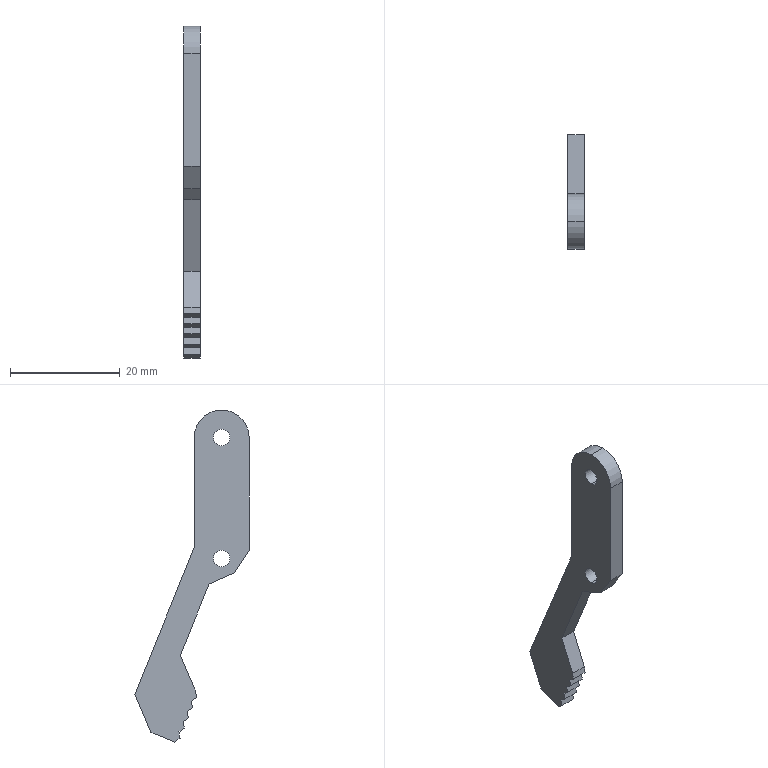Part | SolidWorks | features ICE 3, Extrusion 1 | 1 solid | 28 faces | box 3 x 20.791 x 60.365 mm | volume 1428 mm3 | plane 22 | cylinder 6 | commonest cylinder face diameters 3 x4 10 x2
STEP:
#1=CARTESIAN_POINT('',(3.,5.,-25.5));
#2=VERTEX_POINT('',#1);
#3=CARTESIAN_POINT('',(3.,5.,-28.5));
#4=VERTEX_POINT('',#3);
#5=CARTESIAN_POINT('',(3.,5.,-27.));
#6=DIRECTION('',(1.,0.,0.));
#7=DIRECTION('',(0.,0.,-1.));
#8=AXIS2_PLACEMENT_3D('',#5,#6,#7);
#9=CIRCLE('',#8,1.5);
#10=EDGE_CURVE('',#2,#4,#9,.T.);
#11=ORIENTED_EDGE('',*,*,#10,.T.);
#12=CARTESIAN_POINT('',(0.,5.,-28.5));
#13=VERTEX_POINT('',#12);
#14=CARTESIAN_POINT('',(3.,5.,-28.5));
#15=DIRECTION('',(-1.,0.,0.));
#16=VECTOR('',#15,1000.);
#17=LINE('',#14,#16);
#18=EDGE_CURVE('',#4,#13,#17,.T.);
#19=ORIENTED_EDGE('',*,*,#18,.T.);
#20=CARTESIAN_POINT('',(0.,5.,-25.5));
#21=VERTEX_POINT('',#20);
#22=CARTESIAN_POINT('',(0.,5.,-27.));
#23=DIRECTION('',(1.,0.,0.));
#24=DIRECTION('',(0.,0.,-1.));
#25=AXIS2_PLACEMENT_3D('',#22,#23,#24);
#26=CIRCLE('',#25,1.5);
#27=EDGE_CURVE('',#21,#13,#26,.T.);
#28=ORIENTED_EDGE('',*,*,#27,.F.);
#29=CARTESIAN_POINT('',(3.,5.,-25.5));
#30=DIRECTION('',(-1.,0.,0.));
#31=VECTOR('',#30,1000.);
#32=LINE('',#29,#31);
#33=EDGE_CURVE('',#2,#21,#32,.T.);
#34=ORIENTED_EDGE('',*,*,#33,.F.);
#35=EDGE_LOOP('',(#11,#19,#28,#34));
#36=FACE_OUTER_BOUND('',#35,.T.);
#37=CARTESIAN_POINT('',(3.,5.,-27.));
#38=DIRECTION('',(-1.,0.,0.));
#39=DIRECTION('',(0.,0.,1.));
#40=AXIS2_PLACEMENT_3D('',#37,#38,#39);
#41=CYLINDRICAL_SURFACE('',#40,1.5);
#42=ADVANCED_FACE('',(#36),#41,.F.);
#43=CARTESIAN_POINT('',(3.,5.,-3.5));
#44=VERTEX_POINT('',#43);
#45=CARTESIAN_POINT('',(3.,5.,-6.5));
#46=VERTEX_POINT('',#45);
#47=CARTESIAN_POINT('',(3.,5.,-5.));
#48=DIRECTION('',(1.,0.,0.));
#49=DIRECTION('',(0.,0.,-1.));
#50=AXIS2_PLACEMENT_3D('',#47,#48,#49);
#51=CIRCLE('',#50,1.5);
#52=EDGE_CURVE('',#44,#46,#51,.T.);
#53=ORIENTED_EDGE('',*,*,#52,.T.);
#54=CARTESIAN_POINT('',(0.,5.,-6.5));
#55=VERTEX_POINT('',#54);
#56=CARTESIAN_POINT('',(3.,5.,-6.5));
#57=DIRECTION('',(-1.,0.,0.));
#58=VECTOR('',#57,1000.);
#59=LINE('',#56,#58);
#60=EDGE_CURVE('',#46,#55,#59,.T.);
#61=ORIENTED_EDGE('',*,*,#60,.T.);
#62=CARTESIAN_POINT('',(0.,5.,-3.5));
#63=VERTEX_POINT('',#62);
#64=CARTESIAN_POINT('',(0.,5.,-5.));
#65=DIRECTION('',(1.,0.,0.));
#66=DIRECTION('',(0.,0.,-1.));
#67=AXIS2_PLACEMENT_3D('',#64,#65,#66);
#68=CIRCLE('',#67,1.5);
#69=EDGE_CURVE('',#63,#55,#68,.T.);
#70=ORIENTED_EDGE('',*,*,#69,.F.);
#71=CARTESIAN_POINT('',(3.,5.,-3.5));
#72=DIRECTION('',(-1.,0.,0.));
#73=VECTOR('',#72,1000.);
#74=LINE('',#71,#73);
#75=EDGE_CURVE('',#44,#63,#74,.T.);
#76=ORIENTED_EDGE('',*,*,#75,.F.);
#77=EDGE_LOOP('',(#53,#61,#70,#76));
#78=FACE_OUTER_BOUND('',#77,.T.);
#79=CARTESIAN_POINT('',(3.,5.,-5.));
#80=DIRECTION('',(-1.,0.,0.));
#81=DIRECTION('',(0.,0.,1.));
#82=AXIS2_PLACEMENT_3D('',#79,#80,#81);
#83=CYLINDRICAL_SURFACE('',#82,1.5);
#84=ADVANCED_FACE('',(#78),#83,.F.);
#85=CARTESIAN_POINT('',(3.,5.,0.));
#86=VERTEX_POINT('',#85);
#87=CARTESIAN_POINT('',(3.,0.,-5.));
#88=VERTEX_POINT('',#87);
#89=CARTESIAN_POINT('',(3.,5.,-5.));
#90=DIRECTION('',(1.,0.,0.));
#91=DIRECTION('',(0.,0.,-1.));
#92=AXIS2_PLACEMENT_3D('',#89,#90,#91);
#93=CIRCLE('',#92,5.);
#94=EDGE_CURVE('',#86,#88,#93,.T.);
#95=ORIENTED_EDGE('',*,*,#94,.F.);
#96=CARTESIAN_POINT('',(0.,5.,0.));
#97=VERTEX_POINT('',#96);
#98=CARTESIAN_POINT('',(3.,5.,0.));
#99=DIRECTION('',(-1.,0.,0.));
#100=VECTOR('',#99,1000.);
#101=LINE('',#98,#100);
#102=EDGE_CURVE('',#86,#97,#101,.T.);
#103=ORIENTED_EDGE('',*,*,#102,.T.);
#104=CARTESIAN_POINT('',(0.,0.,-5.));
#105=VERTEX_POINT('',#104);
#106=CARTESIAN_POINT('',(0.,5.,-5.));
#107=DIRECTION('',(1.,0.,0.));
#108=DIRECTION('',(0.,0.,-1.));
#109=AXIS2_PLACEMENT_3D('',#106,#107,#108);
#110=CIRCLE('',#109,5.);
#111=EDGE_CURVE('',#97,#105,#110,.T.);
#112=ORIENTED_EDGE('',*,*,#111,.T.);
#113=CARTESIAN_POINT('',(3.,0.,-5.));
#114=DIRECTION('',(-1.,0.,0.));
#115=VECTOR('',#114,1000.);
#116=LINE('',#113,#115);
#117=EDGE_CURVE('',#88,#105,#116,.T.);
#118=ORIENTED_EDGE('',*,*,#117,.F.);
#119=EDGE_LOOP('',(#95,#103,#112,#118));
#120=FACE_OUTER_BOUND('',#119,.T.);
#121=CARTESIAN_POINT('',(3.,5.,-5.));
#122=DIRECTION('',(-1.,0.,0.));
#123=DIRECTION('',(0.,0.,1.));
#124=AXIS2_PLACEMENT_3D('',#121,#122,#123);
#125=CYLINDRICAL_SURFACE('',#124,5.);
#126=ADVANCED_FACE('',(#120),#125,.T.);
#127=ORIENTED_EDGE('',*,*,#52,.F.);
#128=CARTESIAN_POINT('',(3.,5.,-5.));
#129=DIRECTION('',(1.,0.,0.));
#130=DIRECTION('',(0.,0.,-1.));
#131=AXIS2_PLACEMENT_3D('',#128,#129,#130);
#132=CIRCLE('',#131,1.5);
#133=EDGE_CURVE('',#46,#44,#132,.T.);
#134=ORIENTED_EDGE('',*,*,#133,.F.);
#135=EDGE_LOOP('',(#127,#134));
#136=FACE_BOUND('',#135,.T.);
#137=ORIENTED_EDGE('',*,*,#10,.F.);
#138=CARTESIAN_POINT('',(3.,5.,-27.));
#139=DIRECTION('',(1.,0.,0.));
#140=DIRECTION('',(0.,0.,-1.));
#141=AXIS2_PLACEMENT_3D('',#138,#139,#140);
#142=CIRCLE('',#141,1.5);
#143=EDGE_CURVE('',#4,#2,#142,.T.);
#144=ORIENTED_EDGE('',*,*,#143,.F.);
#145=EDGE_LOOP('',(#137,#144));
#146=FACE_BOUND('',#145,.T.);
#147=CARTESIAN_POINT('',(3.,12.767,-58.512));
#148=VERTEX_POINT('',#147);
#149=CARTESIAN_POINT('',(3.,12.559,-59.675));
#150=VERTEX_POINT('',#149);
#151=CARTESIAN_POINT('',(3.,22.525,-4.035));
#152=DIRECTION('',(0.,-0.1763,-0.9843));
#153=VECTOR('',#152,1000.);
#154=LINE('',#151,#153);
#155=EDGE_CURVE('',#148,#150,#154,.T.);
#156=ORIENTED_EDGE('',*,*,#155,.T.);
#157=CARTESIAN_POINT('',(3.,13.518,-60.365));
#158=VERTEX_POINT('',#157);
#159=CARTESIAN_POINT('',(3.,-24.007,-33.368));
#160=DIRECTION('',(0.,0.8117,-0.584));
#161=VECTOR('',#160,1000.);
#162=LINE('',#159,#161);
#163=EDGE_CURVE('',#150,#158,#162,.T.);
#164=ORIENTED_EDGE('',*,*,#163,.T.);
#165=CARTESIAN_POINT('',(3.,17.861,-58.606));
#166=VERTEX_POINT('',#165);
#167=CARTESIAN_POINT('',(3.,22.915,-56.558));
#168=DIRECTION('',(0.,0.9268,0.3755));
#169=VECTOR('',#168,1000.);
#170=LINE('',#167,#169);
#171=EDGE_CURVE('',#158,#166,#170,.T.);
#172=ORIENTED_EDGE('',*,*,#171,.T.);
#173=CARTESIAN_POINT('',(3.,20.791,-51.684));
#174=VERTEX_POINT('',#173);
#175=CARTESIAN_POINT('',(3.,36.185,-15.318));
#176=DIRECTION('',(0.,-0.3898,-0.9209));
#177=VECTOR('',#176,1000.);
#178=LINE('',#175,#177);
#179=EDGE_CURVE('',#174,#166,#178,.T.);
#180=ORIENTED_EDGE('',*,*,#179,.F.);
#181=CARTESIAN_POINT('',(3.,10.,-25.051));
#182=VERTEX_POINT('',#181);
#183=CARTESIAN_POINT('',(3.,-0.1287,-0.05214));
#184=DIRECTION('',(0.,-0.3755,0.9268));
#185=VECTOR('',#184,1000.);
#186=LINE('',#183,#185);
#187=EDGE_CURVE('',#174,#182,#186,.T.);
#188=ORIENTED_EDGE('',*,*,#187,.T.);
#189=CARTESIAN_POINT('',(3.,10.,-5.));
#190=VERTEX_POINT('',#189);
#191=CARTESIAN_POINT('',(3.,10.,0.));
#192=DIRECTION('',(0.,0.,-1.));
#193=VECTOR('',#192,1000.);
#194=LINE('',#191,#193);
#195=EDGE_CURVE('',#190,#182,#194,.T.);
#196=ORIENTED_EDGE('',*,*,#195,.F.);
#197=CARTESIAN_POINT('',(3.,5.,-5.));
#198=DIRECTION('',(1.,0.,0.));
#199=DIRECTION('',(0.,0.,-1.));
#200=AXIS2_PLACEMENT_3D('',#197,#198,#199);
#201=CIRCLE('',#200,5.);
#202=EDGE_CURVE('',#190,#86,#201,.T.);
#203=ORIENTED_EDGE('',*,*,#202,.T.);
#204=ORIENTED_EDGE('',*,*,#94,.T.);
#205=CARTESIAN_POINT('',(3.,0.,-25.54));
#206=VERTEX_POINT('',#205);
#207=CARTESIAN_POINT('',(3.,0.,0.));
#208=DIRECTION('',(0.,0.,-1.));
#209=VECTOR('',#208,1000.);
#210=LINE('',#207,#209);
#211=EDGE_CURVE('',#88,#206,#210,.T.);
#212=ORIENTED_EDGE('',*,*,#211,.T.);
#213=CARTESIAN_POINT('',(3.,2.665,-29.584));
#214=VERTEX_POINT('',#213);
#215=CARTESIAN_POINT('',(3.,-11.734,-7.733));
#216=DIRECTION('',(0.,-0.5502,0.835));
#217=VECTOR('',#216,1000.);
#218=LINE('',#215,#217);
#219=EDGE_CURVE('',#214,#206,#218,.T.);
#220=ORIENTED_EDGE('',*,*,#219,.F.);
#221=CARTESIAN_POINT('',(3.,7.096,-31.54));
#222=VERTEX_POINT('',#221);
#223=CARTESIAN_POINT('',(3.,-10.494,-23.775));
#224=DIRECTION('',(0.,-0.9148,0.4038));
#225=VECTOR('',#224,1000.);
#226=LINE('',#223,#225);
#227=EDGE_CURVE('',#222,#214,#226,.T.);
#228=ORIENTED_EDGE('',*,*,#227,.F.);
#229=CARTESIAN_POINT('',(3.,7.263,-31.61));
#230=VERTEX_POINT('',#229);
#231=CARTESIAN_POINT('',(3.,-10.244,-24.199));
#232=DIRECTION('',(0.,-0.9209,0.3898));
#233=VECTOR('',#232,1000.);
#234=LINE('',#231,#233);
#235=EDGE_CURVE('',#230,#222,#234,.T.);
#236=ORIENTED_EDGE('',*,*,#235,.F.);
#237=CARTESIAN_POINT('',(3.,12.52,-44.586));
#238=VERTEX_POINT('',#237);
#239=CARTESIAN_POINT('',(3.,-4.763,-1.93));
#240=DIRECTION('',(0.,0.3755,-0.9268));
#241=VECTOR('',#240,1000.);
#242=LINE('',#239,#241);
#243=EDGE_CURVE('',#230,#238,#242,.T.);
#244=ORIENTED_EDGE('',*,*,#243,.T.);
#245=CARTESIAN_POINT('',(3.,9.763,-51.097));
#246=VERTEX_POINT('',#245);
#247=CARTESIAN_POINT('',(3.,26.623,-11.27));
#248=DIRECTION('',(0.,-0.3898,-0.9209));
#249=VECTOR('',#248,1000.);
#250=LINE('',#247,#249);
#251=EDGE_CURVE('',#238,#246,#250,.T.);
#252=ORIENTED_EDGE('',*,*,#251,.T.);
#253=CARTESIAN_POINT('',(3.,9.555,-52.261));
#254=VERTEX_POINT('',#253);
#255=CARTESIAN_POINT('',(3.,18.328,-3.283));
#256=DIRECTION('',(0.,-0.1763,-0.9843));
#257=VECTOR('',#256,1000.);
#258=LINE('',#255,#257);
#259=EDGE_CURVE('',#246,#254,#258,.T.);
#260=ORIENTED_EDGE('',*,*,#259,.T.);
#261=CARTESIAN_POINT('',(3.,10.514,-52.951));
#262=VERTEX_POINT('',#261);
#263=CARTESIAN_POINT('',(3.,-21.516,-29.907));
#264=DIRECTION('',(0.,0.8117,-0.584));
#265=VECTOR('',#264,1000.);
#266=LINE('',#263,#265);
#267=EDGE_CURVE('',#254,#262,#266,.T.);
#268=ORIENTED_EDGE('',*,*,#267,.T.);
#269=CARTESIAN_POINT('',(3.,10.306,-54.114));
#270=VERTEX_POINT('',#269);
#271=CARTESIAN_POINT('',(3.,19.377,-3.471));
#272=DIRECTION('',(0.,-0.1763,-0.9843));
#273=VECTOR('',#272,1000.);
#274=LINE('',#271,#273);
#275=EDGE_CURVE('',#262,#270,#274,.T.);
#276=ORIENTED_EDGE('',*,*,#275,.T.);
#277=CARTESIAN_POINT('',(3.,11.265,-54.805));
#278=VERTEX_POINT('',#277);
#279=CARTESIAN_POINT('',(3.,-22.139,-30.772));
#280=DIRECTION('',(0.,0.8117,-0.584));
#281=VECTOR('',#280,1000.);
#282=LINE('',#279,#281);
#283=EDGE_CURVE('',#270,#278,#282,.T.);
#284=ORIENTED_EDGE('',*,*,#283,.T.);
#285=CARTESIAN_POINT('',(3.,11.057,-55.968));
#286=VERTEX_POINT('',#285);
#287=CARTESIAN_POINT('',(3.,20.426,-3.659));
#288=DIRECTION('',(0.,-0.1763,-0.9843));
#289=VECTOR('',#288,1000.);
#290=LINE('',#287,#289);
#291=EDGE_CURVE('',#278,#286,#290,.T.);
#292=ORIENTED_EDGE('',*,*,#291,.T.);
#293=CARTESIAN_POINT('',(3.,12.016,-56.658));
#294=VERTEX_POINT('',#293);
#295=CARTESIAN_POINT('',(3.,-22.761,-31.637));
#296=DIRECTION('',(0.,0.8117,-0.584));
#297=VECTOR('',#296,1000.);
#298=LINE('',#295,#297);
#299=EDGE_CURVE('',#286,#294,#298,.T.);
#300=ORIENTED_EDGE('',*,*,#299,.T.);
#301=CARTESIAN_POINT('',(3.,11.808,-57.822));
#302=VERTEX_POINT('',#301);
#303=CARTESIAN_POINT('',(3.,21.476,-3.847));
#304=DIRECTION('',(0.,-0.1763,-0.9843));
#305=VECTOR('',#304,1000.);
#306=LINE('',#303,#305);
#307=EDGE_CURVE('',#294,#302,#306,.T.);
#308=ORIENTED_EDGE('',*,*,#307,.T.);
#309=CARTESIAN_POINT('',(3.,-23.384,-32.503));
#310=DIRECTION('',(0.,0.8117,-0.584));
#311=VECTOR('',#310,1000.);
#312=LINE('',#309,#311);
#313=EDGE_CURVE('',#302,#148,#312,.T.);
#314=ORIENTED_EDGE('',*,*,#313,.T.);
#315=EDGE_LOOP('',(#156,#164,#172,#180,#188,#196,#203,#204,#212,#220,#228,#236,#244,#252,#260,#268,#276,#284,#292,#300,#308,#314));
#316=FACE_OUTER_BOUND('',#315,.T.);
#317=CARTESIAN_POINT('',(3.,0.,0.));
#318=DIRECTION('',(1.,0.,0.));
#319=DIRECTION('',(0.,0.,-1.));
#320=AXIS2_PLACEMENT_3D('',#317,#318,#319);
#321=PLANE('',#320);
#322=ADVANCED_FACE('',(#136,#146,#316),#321,.T.);
#323=ORIENTED_EDGE('',*,*,#69,.T.);
#324=CARTESIAN_POINT('',(0.,5.,-5.));
#325=DIRECTION('',(1.,0.,0.));
#326=DIRECTION('',(0.,0.,-1.));
#327=AXIS2_PLACEMENT_3D('',#324,#325,#326);
#328=CIRCLE('',#327,1.5);
#329=EDGE_CURVE('',#55,#63,#328,.T.);
#330=ORIENTED_EDGE('',*,*,#329,.T.);
#331=EDGE_LOOP('',(#323,#330));
#332=FACE_BOUND('',#331,.T.);
#333=ORIENTED_EDGE('',*,*,#27,.T.);
#334=CARTESIAN_POINT('',(0.,5.,-27.));
#335=DIRECTION('',(1.,0.,0.));
#336=DIRECTION('',(0.,0.,-1.));
#337=AXIS2_PLACEMENT_3D('',#334,#335,#336);
#338=CIRCLE('',#337,1.5);
#339=EDGE_CURVE('',#13,#21,#338,.T.);
#340=ORIENTED_EDGE('',*,*,#339,.T.);
#341=EDGE_LOOP('',(#333,#340));
#342=FACE_BOUND('',#341,.T.);
#343=CARTESIAN_POINT('',(0.,12.559,-59.675));
#344=VERTEX_POINT('',#343);
#345=CARTESIAN_POINT('',(0.,13.518,-60.365));
#346=VERTEX_POINT('',#345);
#347=CARTESIAN_POINT('',(0.,-24.007,-33.368));
#348=DIRECTION('',(0.,0.8117,-0.584));
#349=VECTOR('',#348,1000.);
#350=LINE('',#347,#349);
#351=EDGE_CURVE('',#344,#346,#350,.T.);
#352=ORIENTED_EDGE('',*,*,#351,.F.);
#353=CARTESIAN_POINT('',(0.,12.767,-58.512));
#354=VERTEX_POINT('',#353);
#355=CARTESIAN_POINT('',(0.,22.525,-4.035));
#356=DIRECTION('',(0.,-0.1763,-0.9843));
#357=VECTOR('',#356,1000.);
#358=LINE('',#355,#357);
#359=EDGE_CURVE('',#354,#344,#358,.T.);
#360=ORIENTED_EDGE('',*,*,#359,.F.);
#361=CARTESIAN_POINT('',(0.,11.808,-57.822));
#362=VERTEX_POINT('',#361);
#363=CARTESIAN_POINT('',(0.,-23.384,-32.503));
#364=DIRECTION('',(0.,0.8117,-0.584));
#365=VECTOR('',#364,1000.);
#366=LINE('',#363,#365);
#367=EDGE_CURVE('',#362,#354,#366,.T.);
#368=ORIENTED_EDGE('',*,*,#367,.F.);
#369=CARTESIAN_POINT('',(0.,12.016,-56.658));
#370=VERTEX_POINT('',#369);
#371=CARTESIAN_POINT('',(0.,21.476,-3.847));
#372=DIRECTION('',(0.,-0.1763,-0.9843));
#373=VECTOR('',#372,1000.);
#374=LINE('',#371,#373);
#375=EDGE_CURVE('',#370,#362,#374,.T.);
#376=ORIENTED_EDGE('',*,*,#375,.F.);
#377=CARTESIAN_POINT('',(0.,11.057,-55.968));
#378=VERTEX_POINT('',#377);
#379=CARTESIAN_POINT('',(0.,-22.761,-31.637));
#380=DIRECTION('',(0.,0.8117,-0.584));
#381=VECTOR('',#380,1000.);
#382=LINE('',#379,#381);
#383=EDGE_CURVE('',#378,#370,#382,.T.);
#384=ORIENTED_EDGE('',*,*,#383,.F.);
#385=CARTESIAN_POINT('',(0.,11.265,-54.805));
#386=VERTEX_POINT('',#385);
#387=CARTESIAN_POINT('',(0.,20.426,-3.659));
#388=DIRECTION('',(0.,-0.1763,-0.9843));
#389=VECTOR('',#388,1000.);
#390=LINE('',#387,#389);
#391=EDGE_CURVE('',#386,#378,#390,.T.);
#392=ORIENTED_EDGE('',*,*,#391,.F.);
#393=CARTESIAN_POINT('',(0.,10.306,-54.114));
#394=VERTEX_POINT('',#393);
#395=CARTESIAN_POINT('',(0.,-22.139,-30.772));
#396=DIRECTION('',(0.,0.8117,-0.584));
#397=VECTOR('',#396,1000.);
#398=LINE('',#395,#397);
#399=EDGE_CURVE('',#394,#386,#398,.T.);
#400=ORIENTED_EDGE('',*,*,#399,.F.);
#401=CARTESIAN_POINT('',(0.,10.514,-52.951));
#402=VERTEX_POINT('',#401);
#403=CARTESIAN_POINT('',(0.,19.377,-3.471));
#404=DIRECTION('',(0.,-0.1763,-0.9843));
#405=VECTOR('',#404,1000.);
#406=LINE('',#403,#405);
#407=EDGE_CURVE('',#402,#394,#406,.T.);
#408=ORIENTED_EDGE('',*,*,#407,.F.);
#409=CARTESIAN_POINT('',(0.,9.555,-52.261));
#410=VERTEX_POINT('',#409);
#411=CARTESIAN_POINT('',(0.,-21.516,-29.907));
#412=DIRECTION('',(0.,0.8117,-0.584));
#413=VECTOR('',#412,1000.);
#414=LINE('',#411,#413);
#415=EDGE_CURVE('',#410,#402,#414,.T.);
#416=ORIENTED_EDGE('',*,*,#415,.F.);
#417=CARTESIAN_POINT('',(0.,9.763,-51.097));
#418=VERTEX_POINT('',#417);
#419=CARTESIAN_POINT('',(0.,18.328,-3.283));
#420=DIRECTION('',(0.,-0.1763,-0.9843));
#421=VECTOR('',#420,1000.);
#422=LINE('',#419,#421);
#423=EDGE_CURVE('',#418,#410,#422,.T.);
#424=ORIENTED_EDGE('',*,*,#423,.F.);
#425=CARTESIAN_POINT('',(0.,12.52,-44.586));
#426=VERTEX_POINT('',#425);
#427=CARTESIAN_POINT('',(0.,26.623,-11.27));
#428=DIRECTION('',(0.,-0.3898,-0.9209));
#429=VECTOR('',#428,1000.);
#430=LINE('',#427,#429);
#431=EDGE_CURVE('',#426,#418,#430,.T.);
#432=ORIENTED_EDGE('',*,*,#431,.F.);
#433=CARTESIAN_POINT('',(0.,7.263,-31.61));
#434=VERTEX_POINT('',#433);
#435=CARTESIAN_POINT('',(0.,-4.763,-1.93));
#436=DIRECTION('',(0.,0.3755,-0.9268));
#437=VECTOR('',#436,1000.);
#438=LINE('',#435,#437);
#439=EDGE_CURVE('',#434,#426,#438,.T.);
#440=ORIENTED_EDGE('',*,*,#439,.F.);
#441=CARTESIAN_POINT('',(0.,7.096,-31.54));
#442=VERTEX_POINT('',#441);
#443=CARTESIAN_POINT('',(0.,-10.244,-24.199));
#444=DIRECTION('',(0.,-0.9209,0.3898));
#445=VECTOR('',#444,1000.);
#446=LINE('',#443,#445);
#447=EDGE_CURVE('',#434,#442,#446,.T.);
#448=ORIENTED_EDGE('',*,*,#447,.T.);
#449=CARTESIAN_POINT('',(0.,2.665,-29.584));
#450=VERTEX_POINT('',#449);
#451=CARTESIAN_POINT('',(0.,-10.494,-23.775));
#452=DIRECTION('',(0.,-0.9148,0.4038));
#453=VECTOR('',#452,1000.);
#454=LINE('',#451,#453);
#455=EDGE_CURVE('',#442,#450,#454,.T.);
#456=ORIENTED_EDGE('',*,*,#455,.T.);
#457=CARTESIAN_POINT('',(0.,0.,-25.54));
#458=VERTEX_POINT('',#457);
#459=CARTESIAN_POINT('',(0.,-11.734,-7.733));
#460=DIRECTION('',(0.,-0.5502,0.835));
#461=VECTOR('',#460,1000.);
#462=LINE('',#459,#461);
#463=EDGE_CURVE('',#450,#458,#462,.T.);
#464=ORIENTED_EDGE('',*,*,#463,.T.);
#465=CARTESIAN_POINT('',(0.,0.,0.));
#466=DIRECTION('',(0.,0.,-1.));
#467=VECTOR('',#466,1000.);
#468=LINE('',#465,#467);
#469=EDGE_CURVE('',#105,#458,#468,.T.);
#470=ORIENTED_EDGE('',*,*,#469,.F.);
#471=ORIENTED_EDGE('',*,*,#111,.F.);
#472=CARTESIAN_POINT('',(0.,10.,-5.));
#473=VERTEX_POINT('',#472);
#474=CARTESIAN_POINT('',(0.,5.,-5.));
#475=DIRECTION('',(1.,0.,0.));
#476=DIRECTION('',(0.,0.,-1.));
#477=AXIS2_PLACEMENT_3D('',#474,#475,#476);
#478=CIRCLE('',#477,5.);
#479=EDGE_CURVE('',#473,#97,#478,.T.);
#480=ORIENTED_EDGE('',*,*,#479,.F.);
#481=CARTESIAN_POINT('',(0.,10.,-25.051));
#482=VERTEX_POINT('',#481);
#483=CARTESIAN_POINT('',(0.,10.,0.));
#484=DIRECTION('',(0.,0.,-1.));
#485=VECTOR('',#484,1000.);
#486=LINE('',#483,#485);
#487=EDGE_CURVE('',#473,#482,#486,.T.);
#488=ORIENTED_EDGE('',*,*,#487,.T.);
#489=CARTESIAN_POINT('',(0.,20.791,-51.684));
#490=VERTEX_POINT('',#489);
#491=CARTESIAN_POINT('',(0.,-0.1287,-0.05214));
#492=DIRECTION('',(0.,-0.3755,0.9268));
#493=VECTOR('',#492,1000.);
#494=LINE('',#491,#493);
#495=EDGE_CURVE('',#490,#482,#494,.T.);
#496=ORIENTED_EDGE('',*,*,#495,.F.);
#497=CARTESIAN_POINT('',(0.,17.861,-58.606));
#498=VERTEX_POINT('',#497);
#499=CARTESIAN_POINT('',(0.,36.185,-15.318));
#500=DIRECTION('',(0.,-0.3898,-0.9209));
#501=VECTOR('',#500,1000.);
#502=LINE('',#499,#501);
#503=EDGE_CURVE('',#490,#498,#502,.T.);
#504=ORIENTED_EDGE('',*,*,#503,.T.);
#505=CARTESIAN_POINT('',(0.,22.915,-56.558));
#506=DIRECTION('',(0.,0.9268,0.3755));
#507=VECTOR('',#506,1000.);
#508=LINE('',#505,#507);
#509=EDGE_CURVE('',#346,#498,#508,.T.);
#510=ORIENTED_EDGE('',*,*,#509,.F.);
#511=EDGE_LOOP('',(#352,#360,#368,#376,#384,#392,#400,#408,#416,#424,#432,#440,#448,#456,#464,#470,#471,#480,#488,#496,#504,#510));
#512=FACE_OUTER_BOUND('',#511,.T.);
#513=CARTESIAN_POINT('',(0.,0.,0.));
#514=DIRECTION('',(1.,0.,0.));
#515=DIRECTION('',(0.,0.,-1.));
#516=AXIS2_PLACEMENT_3D('',#513,#514,#515);
#517=PLANE('',#516);
#518=ADVANCED_FACE('',(#332,#342,#512),#517,.F.);
#519=ORIENTED_EDGE('',*,*,#171,.F.);
#520=CARTESIAN_POINT('',(-7.,13.518,-60.365));
#521=DIRECTION('',(1.,0.,0.));
#522=VECTOR('',#521,1000.);
#523=LINE('',#520,#522);
#524=EDGE_CURVE('',#346,#158,#523,.T.);
#525=ORIENTED_EDGE('',*,*,#524,.F.);
#526=ORIENTED_EDGE('',*,*,#509,.T.);
#527=CARTESIAN_POINT('',(0.,17.861,-58.606));
#528=DIRECTION('',(1.,0.,0.));
#529=VECTOR('',#528,1000.);
#530=LINE('',#527,#529);
#531=EDGE_CURVE('',#498,#166,#530,.T.);
#532=ORIENTED_EDGE('',*,*,#531,.T.);
#533=EDGE_LOOP('',(#519,#525,#526,#532));
#534=FACE_OUTER_BOUND('',#533,.T.);
#535=CARTESIAN_POINT('',(0.,22.915,-56.558));
#536=DIRECTION('',(0.,0.3755,-0.9268));
#537=DIRECTION('',(0.,0.9268,0.3755));
#538=AXIS2_PLACEMENT_3D('',#535,#536,#537);
#539=PLANE('',#538);
#540=ADVANCED_FACE('',(#534),#539,.T.);
#541=CARTESIAN_POINT('',(0.,10.,-25.051));
#542=DIRECTION('',(1.,0.,0.));
#543=VECTOR('',#542,1000.);
#544=LINE('',#541,#543);
#545=EDGE_CURVE('',#482,#182,#544,.T.);
#546=ORIENTED_EDGE('',*,*,#545,.F.);
#547=ORIENTED_EDGE('',*,*,#487,.F.);
#548=CARTESIAN_POINT('',(3.,10.,-5.));
#549=DIRECTION('',(-1.,0.,0.));
#550=VECTOR('',#549,1000.);
#551=LINE('',#548,#550);
#552=EDGE_CURVE('',#190,#473,#551,.T.);
#553=ORIENTED_EDGE('',*,*,#552,.F.);
#554=ORIENTED_EDGE('',*,*,#195,.T.);
#555=EDGE_LOOP('',(#546,#547,#553,#554));
#556=FACE_OUTER_BOUND('',#555,.T.);
#557=CARTESIAN_POINT('',(3.,10.,0.));
#558=DIRECTION('',(0.,1.,0.));
#559=DIRECTION('',(0.,0.,1.));
#560=AXIS2_PLACEMENT_3D('',#557,#558,#559);
#561=PLANE('',#560);
#562=ADVANCED_FACE('',(#556),#561,.T.);
#563=ORIENTED_EDGE('',*,*,#102,.F.);
#564=ORIENTED_EDGE('',*,*,#202,.F.);
#565=ORIENTED_EDGE('',*,*,#552,.T.);
#566=ORIENTED_EDGE('',*,*,#479,.T.);
#567=EDGE_LOOP('',(#563,#564,#565,#566));
#568=FACE_OUTER_BOUND('',#567,.T.);
#569=CARTESIAN_POINT('',(3.,5.,-5.));
#570=DIRECTION('',(-1.,0.,0.));
#571=DIRECTION('',(0.,0.,1.));
#572=AXIS2_PLACEMENT_3D('',#569,#570,#571);
#573=CYLINDRICAL_SURFACE('',#572,5.);
#574=ADVANCED_FACE('',(#568),#573,.T.);
#575=ORIENTED_EDGE('',*,*,#469,.T.);
#576=CARTESIAN_POINT('',(-7.,0.,-25.54));
#577=DIRECTION('',(1.,0.,0.));
#578=VECTOR('',#577,1000.);
#579=LINE('',#576,#578);
#580=EDGE_CURVE('',#458,#206,#579,.T.);
#581=ORIENTED_EDGE('',*,*,#580,.T.);
#582=ORIENTED_EDGE('',*,*,#211,.F.);
#583=ORIENTED_EDGE('',*,*,#117,.T.);
#584=EDGE_LOOP('',(#575,#581,#582,#583));
#585=FACE_OUTER_BOUND('',#584,.T.);
#586=CARTESIAN_POINT('',(3.,0.,0.));
#587=DIRECTION('',(0.,1.,0.));
#588=DIRECTION('',(0.,0.,1.));
#589=AXIS2_PLACEMENT_3D('',#586,#587,#588);
#590=PLANE('',#589);
#591=ADVANCED_FACE('',(#585),#590,.F.);
#592=ORIENTED_EDGE('',*,*,#60,.F.);
#593=ORIENTED_EDGE('',*,*,#133,.T.);
#594=ORIENTED_EDGE('',*,*,#75,.T.);
#595=ORIENTED_EDGE('',*,*,#329,.F.);
#596=EDGE_LOOP('',(#592,#593,#594,#595));
#597=FACE_OUTER_BOUND('',#596,.T.);
#598=CARTESIAN_POINT('',(3.,5.,-5.));
#599=DIRECTION('',(-1.,0.,0.));
#600=DIRECTION('',(0.,0.,1.));
#601=AXIS2_PLACEMENT_3D('',#598,#599,#600);
#602=CYLINDRICAL_SURFACE('',#601,1.5);
#603=ADVANCED_FACE('',(#597),#602,.F.);
#604=ORIENTED_EDGE('',*,*,#18,.F.);
#605=ORIENTED_EDGE('',*,*,#143,.T.);
#606=ORIENTED_EDGE('',*,*,#33,.T.);
#607=ORIENTED_EDGE('',*,*,#339,.F.);
#608=EDGE_LOOP('',(#604,#605,#606,#607));
#609=FACE_OUTER_BOUND('',#608,.T.);
#610=CARTESIAN_POINT('',(3.,5.,-27.));
#611=DIRECTION('',(-1.,0.,0.));
#612=DIRECTION('',(0.,0.,1.));
#613=AXIS2_PLACEMENT_3D('',#610,#611,#612);
#614=CYLINDRICAL_SURFACE('',#613,1.5);
#615=ADVANCED_FACE('',(#609),#614,.F.);
#616=ORIENTED_EDGE('',*,*,#243,.F.);
#617=CARTESIAN_POINT('',(0.,7.263,-31.61));
#618=DIRECTION('',(1.,0.,0.));
#619=VECTOR('',#618,1000.);
#620=LINE('',#617,#619);
#621=EDGE_CURVE('',#434,#230,#620,.T.);
#622=ORIENTED_EDGE('',*,*,#621,.F.);
#623=ORIENTED_EDGE('',*,*,#439,.T.);
#624=CARTESIAN_POINT('',(0.,12.52,-44.586));
#625=DIRECTION('',(1.,0.,0.));
#626=VECTOR('',#625,1000.);
#627=LINE('',#624,#626);
#628=EDGE_CURVE('',#426,#238,#627,.T.);
#629=ORIENTED_EDGE('',*,*,#628,.T.);
#630=EDGE_LOOP('',(#616,#622,#623,#629));
#631=FACE_OUTER_BOUND('',#630,.T.);
#632=CARTESIAN_POINT('',(0.,-4.763,-1.93));
#633=DIRECTION('',(0.,-0.9268,-0.3755));
#634=DIRECTION('',(0.,0.3755,-0.9268));
#635=AXIS2_PLACEMENT_3D('',#632,#633,#634);
#636=PLANE('',#635);
#637=ADVANCED_FACE('',(#631),#636,.T.);
#638=ORIENTED_EDGE('',*,*,#235,.T.);
#639=CARTESIAN_POINT('',(0.,7.096,-31.54));
#640=DIRECTION('',(1.,0.,0.));
#641=VECTOR('',#640,1000.);
#642=LINE('',#639,#641);
#643=EDGE_CURVE('',#442,#222,#642,.T.);
#644=ORIENTED_EDGE('',*,*,#643,.F.);
#645=ORIENTED_EDGE('',*,*,#447,.F.);
#646=ORIENTED_EDGE('',*,*,#621,.T.);
#647=EDGE_LOOP('',(#638,#644,#645,#646));
#648=FACE_OUTER_BOUND('',#647,.T.);
#649=CARTESIAN_POINT('',(0.,-10.244,-24.199));
#650=DIRECTION('',(0.,0.3898,0.9209));
#651=DIRECTION('',(0.,-0.9209,0.3898));
#652=AXIS2_PLACEMENT_3D('',#649,#650,#651);
#653=PLANE('',#652);
#654=ADVANCED_FACE('',(#648),#653,.F.);
#655=CARTESIAN_POINT('',(0.,20.791,-51.684));
#656=DIRECTION('',(1.,0.,0.));
#657=VECTOR('',#656,1000.);
#658=LINE('',#655,#657);
#659=EDGE_CURVE('',#490,#174,#658,.T.);
#660=ORIENTED_EDGE('',*,*,#659,.F.);
#661=ORIENTED_EDGE('',*,*,#495,.T.);
#662=ORIENTED_EDGE('',*,*,#545,.T.);
#663=ORIENTED_EDGE('',*,*,#187,.F.);
#664=EDGE_LOOP('',(#660,#661,#662,#663));
#665=FACE_OUTER_BOUND('',#664,.T.);
#666=CARTESIAN_POINT('',(0.,-0.1287,-0.05214));
#667=DIRECTION('',(0.,0.9268,0.3755));
#668=DIRECTION('',(0.,-0.3755,0.9268));
#669=AXIS2_PLACEMENT_3D('',#666,#667,#668);
#670=PLANE('',#669);
#671=ADVANCED_FACE('',(#665),#670,.T.);
#672=ORIENTED_EDGE('',*,*,#251,.F.);
#673=ORIENTED_EDGE('',*,*,#628,.F.);
#674=ORIENTED_EDGE('',*,*,#431,.T.);
#675=CARTESIAN_POINT('',(0.,9.763,-51.097));
#676=DIRECTION('',(1.,0.,0.));
#677=VECTOR('',#676,1000.);
#678=LINE('',#675,#677);
#679=EDGE_CURVE('',#418,#246,#678,.T.);
#680=ORIENTED_EDGE('',*,*,#679,.T.);
#681=EDGE_LOOP('',(#672,#673,#674,#680));
#682=FACE_OUTER_BOUND('',#681,.T.);
#683=CARTESIAN_POINT('',(0.,26.623,-11.27));
#684=DIRECTION('',(0.,-0.9209,0.3898));
#685=DIRECTION('',(0.,-0.3898,-0.9209));
#686=AXIS2_PLACEMENT_3D('',#683,#684,#685);
#687=PLANE('',#686);
#688=ADVANCED_FACE('',(#682),#687,.T.);
#689=ORIENTED_EDGE('',*,*,#179,.T.);
#690=ORIENTED_EDGE('',*,*,#531,.F.);
#691=ORIENTED_EDGE('',*,*,#503,.F.);
#692=ORIENTED_EDGE('',*,*,#659,.T.);
#693=EDGE_LOOP('',(#689,#690,#691,#692));
#694=FACE_OUTER_BOUND('',#693,.T.);
#695=CARTESIAN_POINT('',(0.,36.185,-15.318));
#696=DIRECTION('',(0.,-0.9209,0.3898));
#697=DIRECTION('',(0.,-0.3898,-0.9209));
#698=AXIS2_PLACEMENT_3D('',#695,#696,#697);
#699=PLANE('',#698);
#700=ADVANCED_FACE('',(#694),#699,.F.);
#701=CARTESIAN_POINT('',(-7.,2.665,-29.584));
#702=DIRECTION('',(1.,0.,0.));
#703=VECTOR('',#702,1000.);
#704=LINE('',#701,#703);
#705=EDGE_CURVE('',#450,#214,#704,.T.);
#706=ORIENTED_EDGE('',*,*,#705,.T.);
#707=ORIENTED_EDGE('',*,*,#219,.T.);
#708=ORIENTED_EDGE('',*,*,#580,.F.);
#709=ORIENTED_EDGE('',*,*,#463,.F.);
#710=EDGE_LOOP('',(#706,#707,#708,#709));
#711=FACE_OUTER_BOUND('',#710,.T.);
#712=CARTESIAN_POINT('',(-7.,-11.734,-7.733));
#713=DIRECTION('',(0.,0.835,0.5502));
#714=DIRECTION('',(0.,-0.5502,0.835));
#715=AXIS2_PLACEMENT_3D('',#712,#713,#714);
#716=PLANE('',#715);
#717=ADVANCED_FACE('',(#711),#716,.F.);
#718=ORIENTED_EDGE('',*,*,#643,.T.);
#719=ORIENTED_EDGE('',*,*,#227,.T.);
#720=ORIENTED_EDGE('',*,*,#705,.F.);
#721=ORIENTED_EDGE('',*,*,#455,.F.);
#722=EDGE_LOOP('',(#718,#719,#720,#721));
#723=FACE_OUTER_BOUND('',#722,.T.);
#724=CARTESIAN_POINT('',(-7.,-10.494,-23.775));
#725=DIRECTION('',(0.,0.4038,0.9148));
#726=DIRECTION('',(0.,-0.9148,0.4038));
#727=AXIS2_PLACEMENT_3D('',#724,#725,#726);
#728=PLANE('',#727);
#729=ADVANCED_FACE('',(#723),#728,.F.);
#730=ORIENTED_EDGE('',*,*,#423,.T.);
#731=CARTESIAN_POINT('',(-7.,9.555,-52.261));
#732=DIRECTION('',(1.,0.,0.));
#733=VECTOR('',#732,1000.);
#734=LINE('',#731,#733);
#735=EDGE_CURVE('',#410,#254,#734,.T.);
#736=ORIENTED_EDGE('',*,*,#735,.T.);
#737=ORIENTED_EDGE('',*,*,#259,.F.);
#738=ORIENTED_EDGE('',*,*,#679,.F.);
#739=EDGE_LOOP('',(#730,#736,#737,#738));
#740=FACE_OUTER_BOUND('',#739,.T.);
#741=CARTESIAN_POINT('',(-7.,18.328,-3.283));
#742=DIRECTION('',(0.,-0.9843,0.1763));
#743=DIRECTION('',(0.,-0.1763,-0.9843));
#744=AXIS2_PLACEMENT_3D('',#741,#742,#743);
#745=PLANE('',#744);
#746=ADVANCED_FACE('',(#740),#745,.T.);
#747=ORIENTED_EDGE('',*,*,#407,.T.);
#748=CARTESIAN_POINT('',(-7.,10.306,-54.114));
#749=DIRECTION('',(1.,0.,0.));
#750=VECTOR('',#749,1000.);
#751=LINE('',#748,#750);
#752=EDGE_CURVE('',#394,#270,#751,.T.);
#753=ORIENTED_EDGE('',*,*,#752,.T.);
#754=ORIENTED_EDGE('',*,*,#275,.F.);
#755=CARTESIAN_POINT('',(-7.,10.514,-52.951));
#756=DIRECTION('',(1.,0.,0.));
#757=VECTOR('',#756,1000.);
#758=LINE('',#755,#757);
#759=EDGE_CURVE('',#402,#262,#758,.T.);
#760=ORIENTED_EDGE('',*,*,#759,.F.);
#761=EDGE_LOOP('',(#747,#753,#754,#760));
#762=FACE_OUTER_BOUND('',#761,.T.);
#763=CARTESIAN_POINT('',(-7.,19.377,-3.471));
#764=DIRECTION('',(0.,-0.9843,0.1763));
#765=DIRECTION('',(0.,-0.1763,-0.9843));
#766=AXIS2_PLACEMENT_3D('',#763,#764,#765);
#767=PLANE('',#766);
#768=ADVANCED_FACE('',(#762),#767,.T.);
#769=ORIENTED_EDGE('',*,*,#415,.T.);
#770=ORIENTED_EDGE('',*,*,#759,.T.);
#771=ORIENTED_EDGE('',*,*,#267,.F.);
#772=ORIENTED_EDGE('',*,*,#735,.F.);
#773=EDGE_LOOP('',(#769,#770,#771,#772));
#774=FACE_OUTER_BOUND('',#773,.T.);
#775=CARTESIAN_POINT('',(-7.,-21.516,-29.907));
#776=DIRECTION('',(0.,-0.584,-0.8117));
#777=DIRECTION('',(0.,0.8117,-0.584));
#778=AXIS2_PLACEMENT_3D('',#775,#776,#777);
#779=PLANE('',#778);
#780=ADVANCED_FACE('',(#774),#779,.T.);
#781=ORIENTED_EDGE('',*,*,#391,.T.);
#782=CARTESIAN_POINT('',(-7.,11.057,-55.968));
#783=DIRECTION('',(1.,0.,0.));
#784=VECTOR('',#783,1000.);
#785=LINE('',#782,#784);
#786=EDGE_CURVE('',#378,#286,#785,.T.);
#787=ORIENTED_EDGE('',*,*,#786,.T.);
#788=ORIENTED_EDGE('',*,*,#291,.F.);
#789=CARTESIAN_POINT('',(-7.,11.265,-54.805));
#790=DIRECTION('',(1.,0.,0.));
#791=VECTOR('',#790,1000.);
#792=LINE('',#789,#791);
#793=EDGE_CURVE('',#386,#278,#792,.T.);
#794=ORIENTED_EDGE('',*,*,#793,.F.);
#795=EDGE_LOOP('',(#781,#787,#788,#794));
#796=FACE_OUTER_BOUND('',#795,.T.);
#797=CARTESIAN_POINT('',(-7.,20.426,-3.659));
#798=DIRECTION('',(0.,-0.9843,0.1763));
#799=DIRECTION('',(0.,-0.1763,-0.9843));
#800=AXIS2_PLACEMENT_3D('',#797,#798,#799);
#801=PLANE('',#800);
#802=ADVANCED_FACE('',(#796),#801,.T.);
#803=ORIENTED_EDGE('',*,*,#399,.T.);
#804=ORIENTED_EDGE('',*,*,#793,.T.);
#805=ORIENTED_EDGE('',*,*,#283,.F.);
#806=ORIENTED_EDGE('',*,*,#752,.F.);
#807=EDGE_LOOP('',(#803,#804,#805,#806));
#808=FACE_OUTER_BOUND('',#807,.T.);
#809=CARTESIAN_POINT('',(-7.,-22.139,-30.772));
#810=DIRECTION('',(0.,-0.584,-0.8117));
#811=DIRECTION('',(0.,0.8117,-0.584));
#812=AXIS2_PLACEMENT_3D('',#809,#810,#811);
#813=PLANE('',#812);
#814=ADVANCED_FACE('',(#808),#813,.T.);
#815=ORIENTED_EDGE('',*,*,#375,.T.);
#816=CARTESIAN_POINT('',(-7.,11.808,-57.822));
#817=DIRECTION('',(1.,0.,0.));
#818=VECTOR('',#817,1000.);
#819=LINE('',#816,#818);
#820=EDGE_CURVE('',#362,#302,#819,.T.);
#821=ORIENTED_EDGE('',*,*,#820,.T.);
#822=ORIENTED_EDGE('',*,*,#307,.F.);
#823=CARTESIAN_POINT('',(-7.,12.016,-56.658));
#824=DIRECTION('',(1.,0.,0.));
#825=VECTOR('',#824,1000.);
#826=LINE('',#823,#825);
#827=EDGE_CURVE('',#370,#294,#826,.T.);
#828=ORIENTED_EDGE('',*,*,#827,.F.);
#829=EDGE_LOOP('',(#815,#821,#822,#828));
#830=FACE_OUTER_BOUND('',#829,.T.);
#831=CARTESIAN_POINT('',(-7.,21.476,-3.847));
#832=DIRECTION('',(0.,-0.9843,0.1763));
#833=DIRECTION('',(0.,-0.1763,-0.9843));
#834=AXIS2_PLACEMENT_3D('',#831,#832,#833);
#835=PLANE('',#834);
#836=ADVANCED_FACE('',(#830),#835,.T.);
#837=ORIENTED_EDGE('',*,*,#383,.T.);
#838=ORIENTED_EDGE('',*,*,#827,.T.);
#839=ORIENTED_EDGE('',*,*,#299,.F.);
#840=ORIENTED_EDGE('',*,*,#786,.F.);
#841=EDGE_LOOP('',(#837,#838,#839,#840));
#842=FACE_OUTER_BOUND('',#841,.T.);
#843=CARTESIAN_POINT('',(-7.,-22.761,-31.637));
#844=DIRECTION('',(0.,-0.584,-0.8117));
#845=DIRECTION('',(0.,0.8117,-0.584));
#846=AXIS2_PLACEMENT_3D('',#843,#844,#845);
#847=PLANE('',#846);
#848=ADVANCED_FACE('',(#842),#847,.T.);
#849=ORIENTED_EDGE('',*,*,#359,.T.);
#850=CARTESIAN_POINT('',(-7.,12.559,-59.675));
#851=DIRECTION('',(1.,0.,0.));
#852=VECTOR('',#851,1000.);
#853=LINE('',#850,#852);
#854=EDGE_CURVE('',#344,#150,#853,.T.);
#855=ORIENTED_EDGE('',*,*,#854,.T.);
#856=ORIENTED_EDGE('',*,*,#155,.F.);
#857=CARTESIAN_POINT('',(-7.,12.767,-58.512));
#858=DIRECTION('',(1.,0.,0.));
#859=VECTOR('',#858,1000.);
#860=LINE('',#857,#859);
#861=EDGE_CURVE('',#354,#148,#860,.T.);
#862=ORIENTED_EDGE('',*,*,#861,.F.);
#863=EDGE_LOOP('',(#849,#855,#856,#862));
#864=FACE_OUTER_BOUND('',#863,.T.);
#865=CARTESIAN_POINT('',(-7.,22.525,-4.035));
#866=DIRECTION('',(0.,-0.9843,0.1763));
#867=DIRECTION('',(0.,-0.1763,-0.9843));
#868=AXIS2_PLACEMENT_3D('',#865,#866,#867);
#869=PLANE('',#868);
#870=ADVANCED_FACE('',(#864),#869,.T.);
#871=ORIENTED_EDGE('',*,*,#367,.T.);
#872=ORIENTED_EDGE('',*,*,#861,.T.);
#873=ORIENTED_EDGE('',*,*,#313,.F.);
#874=ORIENTED_EDGE('',*,*,#820,.F.);
#875=EDGE_LOOP('',(#871,#872,#873,#874));
#876=FACE_OUTER_BOUND('',#875,.T.);
#877=CARTESIAN_POINT('',(-7.,-23.384,-32.503));
#878=DIRECTION('',(0.,-0.584,-0.8117));
#879=DIRECTION('',(0.,0.8117,-0.584));
#880=AXIS2_PLACEMENT_3D('',#877,#878,#879);
#881=PLANE('',#880);
#882=ADVANCED_FACE('',(#876),#881,.T.);
#883=ORIENTED_EDGE('',*,*,#351,.T.);
#884=ORIENTED_EDGE('',*,*,#524,.T.);
#885=ORIENTED_EDGE('',*,*,#163,.F.);
#886=ORIENTED_EDGE('',*,*,#854,.F.);
#887=EDGE_LOOP('',(#883,#884,#885,#886));
#888=FACE_OUTER_BOUND('',#887,.T.);
#889=CARTESIAN_POINT('',(-7.,-24.007,-33.368));
#890=DIRECTION('',(0.,-0.584,-0.8117));
#891=DIRECTION('',(0.,0.8117,-0.584));
#892=AXIS2_PLACEMENT_3D('',#889,#890,#891);
#893=PLANE('',#892);
#894=ADVANCED_FACE('',(#888),#893,.T.);
#895=CLOSED_SHELL('',(#42,#84,#126,#322,#518,#540,#562,#574,#591,#603,#615,#637,#654,#671,#688,#700,#717,#729,#746,#768,#780,#802,#814,#836,#848,#870,#882,#894));
#896=MANIFOLD_SOLID_BREP('',#895);
#897=CARTESIAN_POINT('',(0.,0.,0.));
#898=DIRECTION('',(0.,0.,1.));
#899=DIRECTION('',(1.,0.,0.));
#900=AXIS2_PLACEMENT_3D('',#897,#898,#899);
#901=(LENGTH_UNIT()NAMED_UNIT(*)SI_UNIT(.MILLI.,.METRE.));
#902=UNCERTAINTY_MEASURE_WITH_UNIT(LENGTH_MEASURE(0.00001),#901,'','');
#903=(NAMED_UNIT(*)PLANE_ANGLE_UNIT()SI_UNIT($,.RADIAN.));
#904=(NAMED_UNIT(*)SI_UNIT($,.STERADIAN.)SOLID_ANGLE_UNIT());
#905=(GEOMETRIC_REPRESENTATION_CONTEXT(3)GLOBAL_UNCERTAINTY_ASSIGNED_CONTEXT((#902))GLOBAL_UNIT_ASSIGNED_CONTEXT((#901,#903,#904))REPRESENTATION_CONTEXT('',''));
#906=ADVANCED_BREP_SHAPE_REPRESENTATION('',(#896,#900),#905);